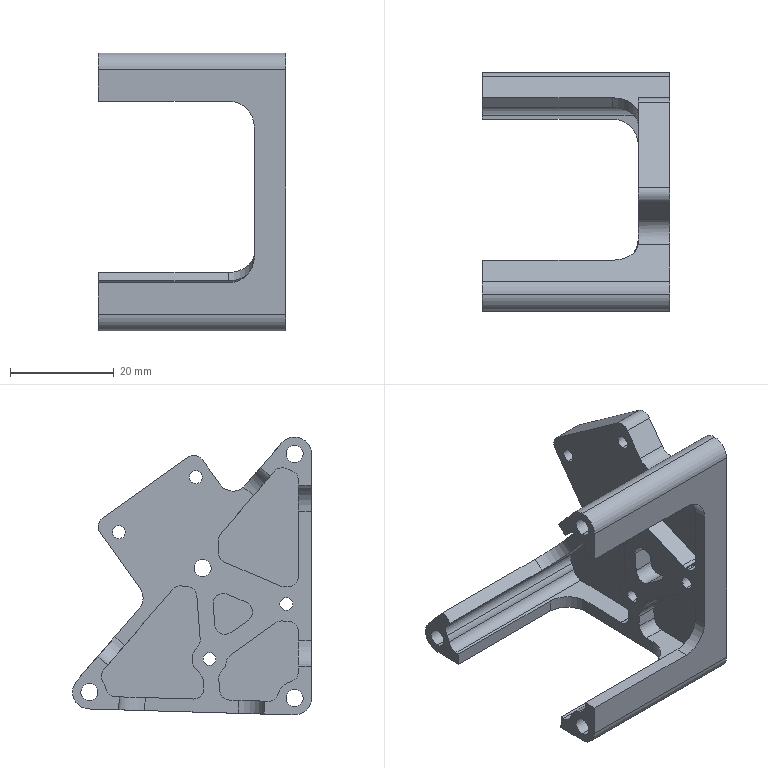Part | SolidWorks | features ICE 9, Fillet 6, HoleWzd 4, Chamfer 1, Extrusion 1 | 1 solid | 104 faces | box 36 x 45.983 x 53.5 mm | volume 11586 mm3 | cylinder 64 | plane 40 | commonest cylinder face diameters 4 x29 2.5 x8 3.3 x8 6.5 x7 10 x6 6.631 x4